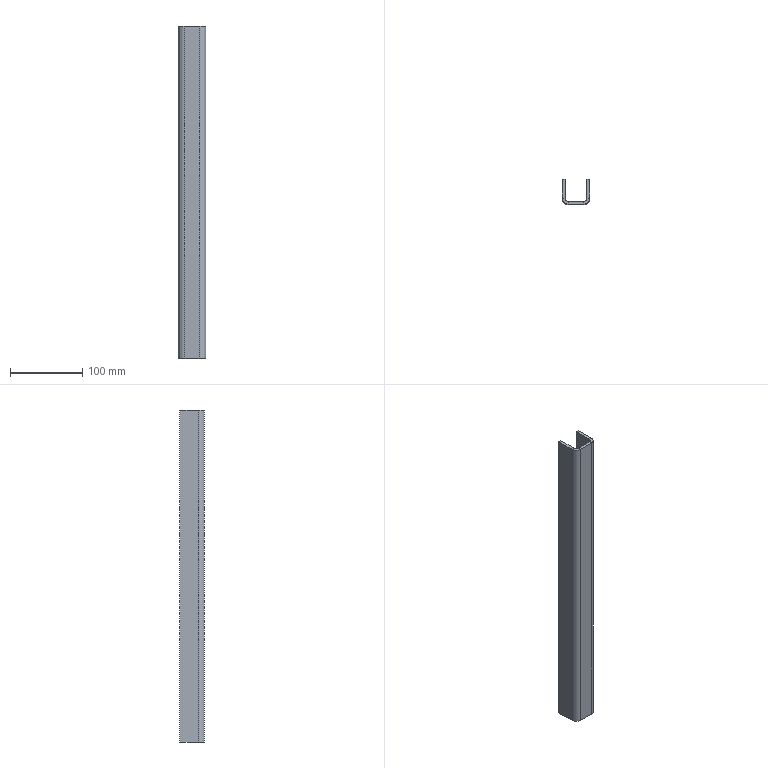Part | STEP file | 17-Reinforcing bent plate 1 | 1 solid | 22 faces | box 38 x 34 x 459 mm | volume 170472 mm3 | plane 18 | cylinder 4 | commonest cylinder face diameters 8 x2 16 x2
STEP:
#1=CARTESIAN_POINT('',(0.,0.,0.));
#2=DIRECTION('',(0.,0.,1.));
#3=DIRECTION('',(1.,0.,0.));
#4=AXIS2_PLACEMENT_3D('',#1,#2,#3);
#5=CARTESIAN_POINT('',(0.,-26.,459.));
#6=VERTEX_POINT('',#5);
#7=CARTESIAN_POINT('',(4.,-26.,459.));
#8=VERTEX_POINT('',#7);
#9=CARTESIAN_POINT('',(0.,-26.,459.));
#10=DIRECTION('',(1.,0.,0.));
#11=VECTOR('',#10,1.);
#12=LINE('',#9,#11);
#13=CARTESIAN_POINT('',(0.,-26.,459.));
#14=DIRECTION('',(0.,0.,1.));
#15=DIRECTION('',(1.,0.,0.));
#16=AXIS2_PLACEMENT_3D('',#13,#14,#15);
#17=PLANE('',#16);
#18=CARTESIAN_POINT('',(0.,0.));
#19=DIRECTION('',(1.,0.));
#20=VECTOR('',#19,1.);
#21=LINE('',#18,#20);
#22=(GEOMETRIC_REPRESENTATION_CONTEXT(2)PARAMETRIC_REPRESENTATION_CONTEXT()REPRESENTATION_CONTEXT('',''));
#23=DEFINITIONAL_REPRESENTATION('',(#21),#22);
#24=PCURVE('',#17,#23);
#25=CARTESIAN_POINT('',(8.,-30.,459.));
#26=DIRECTION('',(0.,0.,1.));
#27=DIRECTION('',(1.,0.,0.));
#28=AXIS2_PLACEMENT_3D('',#25,#26,#27);
#29=PLANE('',#28);
#30=CARTESIAN_POINT('',(-8.,4.));
#31=DIRECTION('',(1.,0.));
#32=VECTOR('',#31,1.);
#33=LINE('',#30,#32);
#34=(GEOMETRIC_REPRESENTATION_CONTEXT(2)PARAMETRIC_REPRESENTATION_CONTEXT()REPRESENTATION_CONTEXT('',''));
#35=DEFINITIONAL_REPRESENTATION('',(#33),#34);
#36=PCURVE('',#29,#35);
#37=SURFACE_CURVE('',#12,(#24,#36),.PCURVE_S1.);
#38=EDGE_CURVE('',#6,#8,#37,.T.);
#39=ORIENTED_EDGE('',*,*,#38,.F.);
#40=CARTESIAN_POINT('',(8.,-34.,459.));
#41=VERTEX_POINT('',#40);
#42=CARTESIAN_POINT('',(8.,-26.,459.));
#43=DIRECTION('',(0.,0.,1.));
#44=DIRECTION('',(-1.,0.,0.));
#45=AXIS2_PLACEMENT_3D('',#42,#43,#44);
#46=CIRCLE('',#45,8.);
#47=CARTESIAN_POINT('',(8.,0.));
#48=DIRECTION('',(-1.,0.));
#49=AXIS2_PLACEMENT_2D('',#47,#48);
#50=CIRCLE('',#49,8.);
#51=(GEOMETRIC_REPRESENTATION_CONTEXT(2)PARAMETRIC_REPRESENTATION_CONTEXT()REPRESENTATION_CONTEXT('',''));
#52=DEFINITIONAL_REPRESENTATION('',(#50),#51);
#53=PCURVE('',#17,#52);
#54=CARTESIAN_POINT('',(8.,-26.,459.));
#55=DIRECTION('',(0.,0.,-1.));
#56=DIRECTION('',(-1.,0.,0.));
#57=AXIS2_PLACEMENT_3D('',#54,#55,#56);
#58=CYLINDRICAL_SURFACE('',#57,8.);
#59=CARTESIAN_POINT('',(6.283,0.));
#60=DIRECTION('',(-1.,0.));
#61=VECTOR('',#60,1.);
#62=LINE('',#59,#61);
#63=(GEOMETRIC_REPRESENTATION_CONTEXT(2)PARAMETRIC_REPRESENTATION_CONTEXT()REPRESENTATION_CONTEXT('',''));
#64=DEFINITIONAL_REPRESENTATION('',(#62),#63);
#65=PCURVE('',#58,#64);
#66=SURFACE_CURVE('',#46,(#53,#65),.PCURVE_S1.);
#67=EDGE_CURVE('',#6,#41,#66,.T.);
#68=ORIENTED_EDGE('',*,*,#67,.T.);
#69=CARTESIAN_POINT('',(8.,-30.,459.));
#70=VERTEX_POINT('',#69);
#71=CARTESIAN_POINT('',(8.,-30.,459.));
#72=DIRECTION('',(0.,-1.,0.));
#73=VECTOR('',#72,1.);
#74=LINE('',#71,#73);
#75=CARTESIAN_POINT('',(8.,-4.));
#76=DIRECTION('',(0.,-1.));
#77=VECTOR('',#76,1.);
#78=LINE('',#75,#77);
#79=(GEOMETRIC_REPRESENTATION_CONTEXT(2)PARAMETRIC_REPRESENTATION_CONTEXT()REPRESENTATION_CONTEXT('',''));
#80=DEFINITIONAL_REPRESENTATION('',(#78),#79);
#81=PCURVE('',#17,#80);
#82=CARTESIAN_POINT('',(34.,-26.,459.));
#83=DIRECTION('',(0.,0.,1.));
#84=DIRECTION('',(1.,0.,0.));
#85=AXIS2_PLACEMENT_3D('',#82,#83,#84);
#86=PLANE('',#85);
#87=CARTESIAN_POINT('',(-26.,-4.));
#88=DIRECTION('',(0.,-1.));
#89=VECTOR('',#88,1.);
#90=LINE('',#87,#89);
#91=(GEOMETRIC_REPRESENTATION_CONTEXT(2)PARAMETRIC_REPRESENTATION_CONTEXT()REPRESENTATION_CONTEXT('',''));
#92=DEFINITIONAL_REPRESENTATION('',(#90),#91);
#93=PCURVE('',#86,#92);
#94=SURFACE_CURVE('',#74,(#81,#93),.PCURVE_S1.);
#95=EDGE_CURVE('',#70,#41,#94,.T.);
#96=ORIENTED_EDGE('',*,*,#95,.F.);
#97=CARTESIAN_POINT('',(8.,-26.,459.));
#98=DIRECTION('',(0.,0.,1.));
#99=DIRECTION('',(1.,0.,0.));
#100=AXIS2_PLACEMENT_3D('',#97,#98,#99);
#101=CIRCLE('',#100,4.);
#102=CARTESIAN_POINT('',(8.,0.));
#103=DIRECTION('',(1.,0.));
#104=AXIS2_PLACEMENT_2D('',#102,#103);
#105=CIRCLE('',#104,4.);
#106=(GEOMETRIC_REPRESENTATION_CONTEXT(2)PARAMETRIC_REPRESENTATION_CONTEXT()REPRESENTATION_CONTEXT('',''));
#107=DEFINITIONAL_REPRESENTATION('',(#105),#106);
#108=PCURVE('',#17,#107);
#109=CARTESIAN_POINT('',(8.,-26.,459.));
#110=DIRECTION('',(0.,0.,-1.));
#111=DIRECTION('',(-1.,0.,0.));
#112=AXIS2_PLACEMENT_3D('',#109,#110,#111);
#113=CYLINDRICAL_SURFACE('',#112,4.);
#114=CARTESIAN_POINT('',(9.425,0.));
#115=DIRECTION('',(-1.,0.));
#116=VECTOR('',#115,1.);
#117=LINE('',#114,#116);
#118=(GEOMETRIC_REPRESENTATION_CONTEXT(2)PARAMETRIC_REPRESENTATION_CONTEXT()REPRESENTATION_CONTEXT('',''));
#119=DEFINITIONAL_REPRESENTATION('',(#117),#118);
#120=PCURVE('',#113,#119);
#121=SURFACE_CURVE('',#101,(#108,#120),.PCURVE_S1.);
#122=EDGE_CURVE('',#8,#70,#121,.T.);
#123=ORIENTED_EDGE('',*,*,#122,.F.);
#124=EDGE_LOOP('',(#39,#68,#96,#123));
#125=FACE_BOUND('',#124,.T.);
#126=ADVANCED_FACE('',(#125),#17,.T.);
#127=CARTESIAN_POINT('',(0.,0.,459.));
#128=VERTEX_POINT('',#127);
#129=CARTESIAN_POINT('',(0.,0.,459.));
#130=DIRECTION('',(0.,-1.,0.));
#131=VECTOR('',#130,1.);
#132=LINE('',#129,#131);
#133=CARTESIAN_POINT('',(-8.,30.));
#134=DIRECTION('',(0.,-1.));
#135=VECTOR('',#134,1.);
#136=LINE('',#133,#135);
#137=(GEOMETRIC_REPRESENTATION_CONTEXT(2)PARAMETRIC_REPRESENTATION_CONTEXT()REPRESENTATION_CONTEXT('',''));
#138=DEFINITIONAL_REPRESENTATION('',(#136),#137);
#139=PCURVE('',#29,#138);
#140=CARTESIAN_POINT('',(0.,0.,459.));
#141=DIRECTION('',(1.,0.,0.));
#142=DIRECTION('',(0.,1.,0.));
#143=AXIS2_PLACEMENT_3D('',#140,#141,#142);
#144=PLANE('',#143);
#145=CARTESIAN_POINT('',(0.,0.));
#146=DIRECTION('',(-1.,0.));
#147=VECTOR('',#146,1.);
#148=LINE('',#145,#147);
#149=(GEOMETRIC_REPRESENTATION_CONTEXT(2)PARAMETRIC_REPRESENTATION_CONTEXT()REPRESENTATION_CONTEXT('',''));
#150=DEFINITIONAL_REPRESENTATION('',(#148),#149);
#151=PCURVE('',#144,#150);
#152=SURFACE_CURVE('',#132,(#139,#151),.PCURVE_S1.);
#153=EDGE_CURVE('',#128,#6,#152,.T.);
#154=ORIENTED_EDGE('',*,*,#153,.T.);
#155=ORIENTED_EDGE('',*,*,#38,.T.);
#156=CARTESIAN_POINT('',(4.,0.,459.));
#157=VERTEX_POINT('',#156);
#158=CARTESIAN_POINT('',(4.,0.,459.));
#159=DIRECTION('',(0.,-1.,0.));
#160=VECTOR('',#159,1.);
#161=LINE('',#158,#160);
#162=CARTESIAN_POINT('',(-4.,30.));
#163=DIRECTION('',(0.,-1.));
#164=VECTOR('',#163,1.);
#165=LINE('',#162,#164);
#166=(GEOMETRIC_REPRESENTATION_CONTEXT(2)PARAMETRIC_REPRESENTATION_CONTEXT()REPRESENTATION_CONTEXT('',''));
#167=DEFINITIONAL_REPRESENTATION('',(#165),#166);
#168=PCURVE('',#29,#167);
#169=CARTESIAN_POINT('',(4.,0.,459.));
#170=DIRECTION('',(1.,0.,0.));
#171=DIRECTION('',(0.,1.,0.));
#172=AXIS2_PLACEMENT_3D('',#169,#170,#171);
#173=PLANE('',#172);
#174=CARTESIAN_POINT('',(0.,0.));
#175=DIRECTION('',(-1.,0.));
#176=VECTOR('',#175,1.);
#177=LINE('',#174,#176);
#178=(GEOMETRIC_REPRESENTATION_CONTEXT(2)PARAMETRIC_REPRESENTATION_CONTEXT()REPRESENTATION_CONTEXT('',''));
#179=DEFINITIONAL_REPRESENTATION('',(#177),#178);
#180=PCURVE('',#173,#179);
#181=SURFACE_CURVE('',#161,(#168,#180),.PCURVE_S1.);
#182=EDGE_CURVE('',#157,#8,#181,.T.);
#183=ORIENTED_EDGE('',*,*,#182,.F.);
#184=CARTESIAN_POINT('',(0.,0.,459.));
#185=DIRECTION('',(1.,0.,0.));
#186=VECTOR('',#185,1.);
#187=LINE('',#184,#186);
#188=CARTESIAN_POINT('',(-8.,30.));
#189=DIRECTION('',(1.,0.));
#190=VECTOR('',#189,1.);
#191=LINE('',#188,#190);
#192=(GEOMETRIC_REPRESENTATION_CONTEXT(2)PARAMETRIC_REPRESENTATION_CONTEXT()REPRESENTATION_CONTEXT('',''));
#193=DEFINITIONAL_REPRESENTATION('',(#191),#192);
#194=PCURVE('',#29,#193);
#195=CARTESIAN_POINT('',(0.,0.,459.));
#196=DIRECTION('',(0.,1.,0.));
#197=DIRECTION('',(-1.,0.,0.));
#198=AXIS2_PLACEMENT_3D('',#195,#196,#197);
#199=PLANE('',#198);
#200=CARTESIAN_POINT('',(0.,0.));
#201=DIRECTION('',(-1.,0.));
#202=VECTOR('',#201,1.);
#203=LINE('',#200,#202);
#204=(GEOMETRIC_REPRESENTATION_CONTEXT(2)PARAMETRIC_REPRESENTATION_CONTEXT()REPRESENTATION_CONTEXT('',''));
#205=DEFINITIONAL_REPRESENTATION('',(#203),#204);
#206=PCURVE('',#199,#205);
#207=SURFACE_CURVE('',#187,(#194,#206),.PCURVE_S1.);
#208=EDGE_CURVE('',#128,#157,#207,.T.);
#209=ORIENTED_EDGE('',*,*,#208,.F.);
#210=EDGE_LOOP('',(#154,#155,#183,#209));
#211=FACE_BOUND('',#210,.T.);
#212=ADVANCED_FACE('',(#211),#29,.T.);
#213=CARTESIAN_POINT('',(8.,-34.,0.));
#214=VERTEX_POINT('',#213);
#215=CARTESIAN_POINT('',(8.,-30.,0.));
#216=VERTEX_POINT('',#215);
#217=CARTESIAN_POINT('',(8.,-34.,0.));
#218=DIRECTION('',(0.,1.,0.));
#219=VECTOR('',#218,1.);
#220=LINE('',#217,#219);
#221=CARTESIAN_POINT('',(8.,-34.,0.));
#222=DIRECTION('',(0.,0.,-1.));
#223=DIRECTION('',(-1.,0.,0.));
#224=AXIS2_PLACEMENT_3D('',#221,#222,#223);
#225=PLANE('',#224);
#226=CARTESIAN_POINT('',(0.,0.));
#227=DIRECTION('',(0.,1.));
#228=VECTOR('',#227,1.);
#229=LINE('',#226,#228);
#230=(GEOMETRIC_REPRESENTATION_CONTEXT(2)PARAMETRIC_REPRESENTATION_CONTEXT()REPRESENTATION_CONTEXT('',''));
#231=DEFINITIONAL_REPRESENTATION('',(#229),#230);
#232=PCURVE('',#225,#231);
#233=CARTESIAN_POINT('',(4.,-26.,0.));
#234=DIRECTION('',(0.,0.,-1.));
#235=DIRECTION('',(-1.,0.,0.));
#236=AXIS2_PLACEMENT_3D('',#233,#234,#235);
#237=PLANE('',#236);
#238=CARTESIAN_POINT('',(-4.,-8.));
#239=DIRECTION('',(0.,1.));
#240=VECTOR('',#239,1.);
#241=LINE('',#238,#240);
#242=(GEOMETRIC_REPRESENTATION_CONTEXT(2)PARAMETRIC_REPRESENTATION_CONTEXT()REPRESENTATION_CONTEXT('',''));
#243=DEFINITIONAL_REPRESENTATION('',(#241),#242);
#244=PCURVE('',#237,#243);
#245=SURFACE_CURVE('',#220,(#232,#244),.PCURVE_S1.);
#246=EDGE_CURVE('',#214,#216,#245,.T.);
#247=ORIENTED_EDGE('',*,*,#246,.F.);
#248=CARTESIAN_POINT('',(0.,-26.,0.));
#249=VERTEX_POINT('',#248);
#250=CARTESIAN_POINT('',(8.,-26.,0.));
#251=DIRECTION('',(0.,0.,1.));
#252=DIRECTION('',(-1.,0.,0.));
#253=AXIS2_PLACEMENT_3D('',#250,#251,#252);
#254=CIRCLE('',#253,8.);
#255=CARTESIAN_POINT('',(8.,8.));
#256=CARTESIAN_POINT('',(8.,-5.856));
#257=CARTESIAN_POINT('',(-4.,1.072));
#258=CARTESIAN_POINT('',(-16.,8.));
#259=CARTESIAN_POINT('',(-4.,14.928));
#260=CARTESIAN_POINT('',(8.,21.856));
#261=CARTESIAN_POINT('',(8.,8.));
#262=(BOUNDED_CURVE()B_SPLINE_CURVE(2,(#255,#256,#257,#258,#259,#260,#261),.UNSPECIFIED.,.T.,.F.)B_SPLINE_CURVE_WITH_KNOTS((1,2,2,2,2,1),(-2.094,0.,2.094,4.189,6.283,8.378),.UNSPECIFIED.)CURVE()GEOMETRIC_REPRESENTATION_ITEM()RATIONAL_B_SPLINE_CURVE((1.,0.5,1.,0.5,1.,0.5,1.))REPRESENTATION_ITEM(''));
#263=(GEOMETRIC_REPRESENTATION_CONTEXT(2)PARAMETRIC_REPRESENTATION_CONTEXT()REPRESENTATION_CONTEXT('',''));
#264=DEFINITIONAL_REPRESENTATION('',(#262),#263);
#265=PCURVE('',#225,#264);
#266=CARTESIAN_POINT('',(6.283,459.));
#267=DIRECTION('',(-1.,0.));
#268=VECTOR('',#267,1.);
#269=LINE('',#266,#268);
#270=(GEOMETRIC_REPRESENTATION_CONTEXT(2)PARAMETRIC_REPRESENTATION_CONTEXT()REPRESENTATION_CONTEXT('',''));
#271=DEFINITIONAL_REPRESENTATION('',(#269),#270);
#272=PCURVE('',#58,#271);
#273=SURFACE_CURVE('',#254,(#265,#272),.PCURVE_S1.);
#274=EDGE_CURVE('',#249,#214,#273,.T.);
#275=ORIENTED_EDGE('',*,*,#274,.F.);
#276=CARTESIAN_POINT('',(4.,-26.,0.));
#277=VERTEX_POINT('',#276);
#278=CARTESIAN_POINT('',(4.,-26.,0.));
#279=DIRECTION('',(-1.,0.,0.));
#280=VECTOR('',#279,1.);
#281=LINE('',#278,#280);
#282=CARTESIAN_POINT('',(4.,8.));
#283=DIRECTION('',(1.,0.));
#284=VECTOR('',#283,1.);
#285=LINE('',#282,#284);
#286=(GEOMETRIC_REPRESENTATION_CONTEXT(2)PARAMETRIC_REPRESENTATION_CONTEXT()REPRESENTATION_CONTEXT('',''));
#287=DEFINITIONAL_REPRESENTATION('',(#285),#286);
#288=PCURVE('',#225,#287);
#289=CARTESIAN_POINT('',(30.,-26.,0.));
#290=DIRECTION('',(0.,0.,1.));
#291=DIRECTION('',(1.,0.,0.));
#292=AXIS2_PLACEMENT_3D('',#289,#290,#291);
#293=PLANE('',#292);
#294=CARTESIAN_POINT('',(-26.,0.));
#295=DIRECTION('',(-1.,0.));
#296=VECTOR('',#295,1.);
#297=LINE('',#294,#296);
#298=(GEOMETRIC_REPRESENTATION_CONTEXT(2)PARAMETRIC_REPRESENTATION_CONTEXT()REPRESENTATION_CONTEXT('',''));
#299=DEFINITIONAL_REPRESENTATION('',(#297),#298);
#300=PCURVE('',#293,#299);
#301=SURFACE_CURVE('',#281,(#288,#300),.PCURVE_S1.);
#302=EDGE_CURVE('',#277,#249,#301,.T.);
#303=ORIENTED_EDGE('',*,*,#302,.F.);
#304=CARTESIAN_POINT('',(8.,-26.,0.));
#305=DIRECTION('',(0.,0.,1.));
#306=DIRECTION('',(1.,0.,0.));
#307=AXIS2_PLACEMENT_3D('',#304,#305,#306);
#308=CIRCLE('',#307,4.);
#309=CARTESIAN_POINT('',(-4.,8.));
#310=CARTESIAN_POINT('',(-4.,14.928));
#311=CARTESIAN_POINT('',(2.,11.464));
#312=CARTESIAN_POINT('',(8.,8.));
#313=CARTESIAN_POINT('',(2.,4.536));
#314=CARTESIAN_POINT('',(-4.,1.072));
#315=CARTESIAN_POINT('',(-4.,8.));
#316=(BOUNDED_CURVE()B_SPLINE_CURVE(2,(#309,#310,#311,#312,#313,#314,#315),.UNSPECIFIED.,.T.,.F.)B_SPLINE_CURVE_WITH_KNOTS((1,2,2,2,2,1),(-2.094,0.,2.094,4.189,6.283,8.378),.UNSPECIFIED.)CURVE()GEOMETRIC_REPRESENTATION_ITEM()RATIONAL_B_SPLINE_CURVE((1.,0.5,1.,0.5,1.,0.5,1.))REPRESENTATION_ITEM(''));
#317=(GEOMETRIC_REPRESENTATION_CONTEXT(2)PARAMETRIC_REPRESENTATION_CONTEXT()REPRESENTATION_CONTEXT('',''));
#318=DEFINITIONAL_REPRESENTATION('',(#316),#317);
#319=PCURVE('',#225,#318);
#320=CARTESIAN_POINT('',(9.425,459.));
#321=DIRECTION('',(-1.,0.));
#322=VECTOR('',#321,1.);
#323=LINE('',#320,#322);
#324=(GEOMETRIC_REPRESENTATION_CONTEXT(2)PARAMETRIC_REPRESENTATION_CONTEXT()REPRESENTATION_CONTEXT('',''));
#325=DEFINITIONAL_REPRESENTATION('',(#323),#324);
#326=PCURVE('',#113,#325);
#327=SURFACE_CURVE('',#308,(#319,#326),.PCURVE_S1.);
#328=EDGE_CURVE('',#277,#216,#327,.T.);
#329=ORIENTED_EDGE('',*,*,#328,.T.);
#330=EDGE_LOOP('',(#247,#275,#303,#329));
#331=FACE_BOUND('',#330,.T.);
#332=ADVANCED_FACE('',(#331),#225,.T.);
#333=CARTESIAN_POINT('',(30.,-34.,0.));
#334=VERTEX_POINT('',#333);
#335=CARTESIAN_POINT('',(0.,-34.,0.));
#336=DIRECTION('',(1.,0.,0.));
#337=VECTOR('',#336,1.);
#338=LINE('',#335,#337);
#339=CARTESIAN_POINT('',(4.,-8.));
#340=DIRECTION('',(-1.,0.));
#341=VECTOR('',#340,1.);
#342=LINE('',#339,#341);
#343=(GEOMETRIC_REPRESENTATION_CONTEXT(2)PARAMETRIC_REPRESENTATION_CONTEXT()REPRESENTATION_CONTEXT('',''));
#344=DEFINITIONAL_REPRESENTATION('',(#342),#343);
#345=PCURVE('',#237,#344);
#346=CARTESIAN_POINT('',(0.,-34.,459.));
#347=DIRECTION('',(0.,1.,0.));
#348=DIRECTION('',(0.,0.,1.));
#349=AXIS2_PLACEMENT_3D('',#346,#347,#348);
#350=PLANE('',#349);
#351=CARTESIAN_POINT('',(-459.,0.));
#352=DIRECTION('',(0.,1.));
#353=VECTOR('',#352,1.);
#354=LINE('',#351,#353);
#355=(GEOMETRIC_REPRESENTATION_CONTEXT(2)PARAMETRIC_REPRESENTATION_CONTEXT()REPRESENTATION_CONTEXT('',''));
#356=DEFINITIONAL_REPRESENTATION('',(#354),#355);
#357=PCURVE('',#350,#356);
#358=SURFACE_CURVE('',#338,(#345,#357),.PCURVE_S1.);
#359=EDGE_CURVE('',#214,#334,#358,.T.);
#360=ORIENTED_EDGE('',*,*,#359,.F.);
#361=ORIENTED_EDGE('',*,*,#246,.T.);
#362=CARTESIAN_POINT('',(30.,-30.,0.));
#363=VERTEX_POINT('',#362);
#364=CARTESIAN_POINT('',(0.,-30.,0.));
#365=DIRECTION('',(1.,0.,0.));
#366=VECTOR('',#365,1.);
#367=LINE('',#364,#366);
#368=CARTESIAN_POINT('',(4.,-4.));
#369=DIRECTION('',(-1.,0.));
#370=VECTOR('',#369,1.);
#371=LINE('',#368,#370);
#372=(GEOMETRIC_REPRESENTATION_CONTEXT(2)PARAMETRIC_REPRESENTATION_CONTEXT()REPRESENTATION_CONTEXT('',''));
#373=DEFINITIONAL_REPRESENTATION('',(#371),#372);
#374=PCURVE('',#237,#373);
#375=CARTESIAN_POINT('',(0.,-30.,459.));
#376=DIRECTION('',(0.,1.,0.));
#377=DIRECTION('',(0.,0.,1.));
#378=AXIS2_PLACEMENT_3D('',#375,#376,#377);
#379=PLANE('',#378);
#380=CARTESIAN_POINT('',(-459.,0.));
#381=DIRECTION('',(0.,1.));
#382=VECTOR('',#381,1.);
#383=LINE('',#380,#382);
#384=(GEOMETRIC_REPRESENTATION_CONTEXT(2)PARAMETRIC_REPRESENTATION_CONTEXT()REPRESENTATION_CONTEXT('',''));
#385=DEFINITIONAL_REPRESENTATION('',(#383),#384);
#386=PCURVE('',#379,#385);
#387=SURFACE_CURVE('',#367,(#374,#386),.PCURVE_S1.);
#388=EDGE_CURVE('',#216,#363,#387,.T.);
#389=ORIENTED_EDGE('',*,*,#388,.T.);
#390=CARTESIAN_POINT('',(30.,-30.,0.));
#391=DIRECTION('',(0.,-1.,0.));
#392=VECTOR('',#391,1.);
#393=LINE('',#390,#392);
#394=CARTESIAN_POINT('',(-26.,-4.));
#395=DIRECTION('',(0.,-1.));
#396=VECTOR('',#395,1.);
#397=LINE('',#394,#396);
#398=(GEOMETRIC_REPRESENTATION_CONTEXT(2)PARAMETRIC_REPRESENTATION_CONTEXT()REPRESENTATION_CONTEXT('',''));
#399=DEFINITIONAL_REPRESENTATION('',(#397),#398);
#400=PCURVE('',#237,#399);
#401=CARTESIAN_POINT('',(38.,-26.,0.));
#402=DIRECTION('',(0.,0.,-1.));
#403=DIRECTION('',(-1.,0.,0.));
#404=AXIS2_PLACEMENT_3D('',#401,#402,#403);
#405=PLANE('',#404);
#406=CARTESIAN_POINT('',(8.,-4.));
#407=DIRECTION('',(0.,-1.));
#408=VECTOR('',#407,1.);
#409=LINE('',#406,#408);
#410=(GEOMETRIC_REPRESENTATION_CONTEXT(2)PARAMETRIC_REPRESENTATION_CONTEXT()REPRESENTATION_CONTEXT('',''));
#411=DEFINITIONAL_REPRESENTATION('',(#409),#410);
#412=PCURVE('',#405,#411);
#413=SURFACE_CURVE('',#393,(#400,#412),.PCURVE_S1.);
#414=EDGE_CURVE('',#363,#334,#413,.T.);
#415=ORIENTED_EDGE('',*,*,#414,.T.);
#416=EDGE_LOOP('',(#360,#361,#389,#415));
#417=FACE_BOUND('',#416,.T.);
#418=ADVANCED_FACE('',(#417),#237,.T.);
#419=CARTESIAN_POINT('',(30.,-34.,459.));
#420=VERTEX_POINT('',#419);
#421=CARTESIAN_POINT('',(30.,-30.,459.));
#422=VERTEX_POINT('',#421);
#423=CARTESIAN_POINT('',(30.,-34.,459.));
#424=DIRECTION('',(0.,1.,0.));
#425=VECTOR('',#424,1.);
#426=LINE('',#423,#425);
#427=CARTESIAN_POINT('',(30.,-34.,459.));
#428=DIRECTION('',(0.,0.,1.));
#429=DIRECTION('',(1.,0.,0.));
#430=AXIS2_PLACEMENT_3D('',#427,#428,#429);
#431=PLANE('',#430);
#432=CARTESIAN_POINT('',(0.,0.));
#433=DIRECTION('',(0.,1.));
#434=VECTOR('',#433,1.);
#435=LINE('',#432,#434);
#436=(GEOMETRIC_REPRESENTATION_CONTEXT(2)PARAMETRIC_REPRESENTATION_CONTEXT()REPRESENTATION_CONTEXT('',''));
#437=DEFINITIONAL_REPRESENTATION('',(#435),#436);
#438=PCURVE('',#431,#437);
#439=CARTESIAN_POINT('',(-4.,-8.));
#440=DIRECTION('',(0.,1.));
#441=VECTOR('',#440,1.);
#442=LINE('',#439,#441);
#443=(GEOMETRIC_REPRESENTATION_CONTEXT(2)PARAMETRIC_REPRESENTATION_CONTEXT()REPRESENTATION_CONTEXT('',''));
#444=DEFINITIONAL_REPRESENTATION('',(#442),#443);
#445=PCURVE('',#86,#444);
#446=SURFACE_CURVE('',#426,(#438,#445),.PCURVE_S1.);
#447=EDGE_CURVE('',#420,#422,#446,.T.);
#448=ORIENTED_EDGE('',*,*,#447,.F.);
#449=CARTESIAN_POINT('',(38.,-26.,459.));
#450=VERTEX_POINT('',#449);
#451=CARTESIAN_POINT('',(30.,-26.,459.));
#452=DIRECTION('',(0.,0.,1.));
#453=DIRECTION('',(-1.,0.,0.));
#454=AXIS2_PLACEMENT_3D('',#451,#452,#453);
#455=CIRCLE('',#454,8.);
#456=CARTESIAN_POINT('',(0.,8.));
#457=DIRECTION('',(-1.,0.));
#458=AXIS2_PLACEMENT_2D('',#456,#457);
#459=CIRCLE('',#458,8.);
#460=(GEOMETRIC_REPRESENTATION_CONTEXT(2)PARAMETRIC_REPRESENTATION_CONTEXT()REPRESENTATION_CONTEXT('',''));
#461=DEFINITIONAL_REPRESENTATION('',(#459),#460);
#462=PCURVE('',#431,#461);
#463=CARTESIAN_POINT('',(30.,-26.,459.));
#464=DIRECTION('',(0.,0.,-1.));
#465=DIRECTION('',(-1.,0.,0.));
#466=AXIS2_PLACEMENT_3D('',#463,#464,#465);
#467=CYLINDRICAL_SURFACE('',#466,8.);
#468=CARTESIAN_POINT('',(6.283,0.));
#469=DIRECTION('',(-1.,0.));
#470=VECTOR('',#469,1.);
#471=LINE('',#468,#470);
#472=(GEOMETRIC_REPRESENTATION_CONTEXT(2)PARAMETRIC_REPRESENTATION_CONTEXT()REPRESENTATION_CONTEXT('',''));
#473=DEFINITIONAL_REPRESENTATION('',(#471),#472);
#474=PCURVE('',#467,#473);
#475=SURFACE_CURVE('',#455,(#462,#474),.PCURVE_S1.);
#476=EDGE_CURVE('',#420,#450,#475,.T.);
#477=ORIENTED_EDGE('',*,*,#476,.T.);
#478=CARTESIAN_POINT('',(34.,-26.,459.));
#479=VERTEX_POINT('',#478);
#480=CARTESIAN_POINT('',(34.,-26.,459.));
#481=DIRECTION('',(1.,0.,0.));
#482=VECTOR('',#481,1.);
#483=LINE('',#480,#482);
#484=CARTESIAN_POINT('',(4.,8.));
#485=DIRECTION('',(1.,0.));
#486=VECTOR('',#485,1.);
#487=LINE('',#484,#486);
#488=(GEOMETRIC_REPRESENTATION_CONTEXT(2)PARAMETRIC_REPRESENTATION_CONTEXT()REPRESENTATION_CONTEXT('',''));
#489=DEFINITIONAL_REPRESENTATION('',(#487),#488);
#490=PCURVE('',#431,#489);
#491=CARTESIAN_POINT('',(30.,-26.,459.));
#492=DIRECTION('',(0.,0.,1.));
#493=DIRECTION('',(1.,0.,0.));
#494=AXIS2_PLACEMENT_3D('',#491,#492,#493);
#495=PLANE('',#494);
#496=CARTESIAN_POINT('',(4.,0.));
#497=DIRECTION('',(1.,0.));
#498=VECTOR('',#497,1.);
#499=LINE('',#496,#498);
#500=(GEOMETRIC_REPRESENTATION_CONTEXT(2)PARAMETRIC_REPRESENTATION_CONTEXT()REPRESENTATION_CONTEXT('',''));
#501=DEFINITIONAL_REPRESENTATION('',(#499),#500);
#502=PCURVE('',#495,#501);
#503=SURFACE_CURVE('',#483,(#490,#502),.PCURVE_S1.);
#504=EDGE_CURVE('',#479,#450,#503,.T.);
#505=ORIENTED_EDGE('',*,*,#504,.F.);
#506=CARTESIAN_POINT('',(30.,-26.,459.));
#507=DIRECTION('',(0.,0.,1.));
#508=DIRECTION('',(1.,0.,0.));
#509=AXIS2_PLACEMENT_3D('',#506,#507,#508);
#510=CIRCLE('',#509,4.);
#511=CARTESIAN_POINT('',(0.,8.));
#512=DIRECTION('',(1.,0.));
#513=AXIS2_PLACEMENT_2D('',#511,#512);
#514=CIRCLE('',#513,4.);
#515=(GEOMETRIC_REPRESENTATION_CONTEXT(2)PARAMETRIC_REPRESENTATION_CONTEXT()REPRESENTATION_CONTEXT('',''));
#516=DEFINITIONAL_REPRESENTATION('',(#514),#515);
#517=PCURVE('',#431,#516);
#518=CARTESIAN_POINT('',(30.,-26.,459.));
#519=DIRECTION('',(0.,0.,-1.));
#520=DIRECTION('',(-1.,0.,0.));
#521=AXIS2_PLACEMENT_3D('',#518,#519,#520);
#522=CYLINDRICAL_SURFACE('',#521,4.);
#523=CARTESIAN_POINT('',(9.425,0.));
#524=DIRECTION('',(-1.,0.));
#525=VECTOR('',#524,1.);
#526=LINE('',#523,#525);
#527=(GEOMETRIC_REPRESENTATION_CONTEXT(2)PARAMETRIC_REPRESENTATION_CONTEXT()REPRESENTATION_CONTEXT('',''));
#528=DEFINITIONAL_REPRESENTATION('',(#526),#527);
#529=PCURVE('',#522,#528);
#530=SURFACE_CURVE('',#510,(#517,#529),.PCURVE_S1.);
#531=EDGE_CURVE('',#422,#479,#530,.T.);
#532=ORIENTED_EDGE('',*,*,#531,.F.);
#533=EDGE_LOOP('',(#448,#477,#505,#532));
#534=FACE_BOUND('',#533,.T.);
#535=ADVANCED_FACE('',(#534),#431,.T.);
#536=CARTESIAN_POINT('',(0.,-34.,459.));
#537=DIRECTION('',(1.,0.,0.));
#538=VECTOR('',#537,1.);
#539=LINE('',#536,#538);
#540=CARTESIAN_POINT('',(-34.,-8.));
#541=DIRECTION('',(1.,0.));
#542=VECTOR('',#541,1.);
#543=LINE('',#540,#542);
#544=(GEOMETRIC_REPRESENTATION_CONTEXT(2)PARAMETRIC_REPRESENTATION_CONTEXT()REPRESENTATION_CONTEXT('',''));
#545=DEFINITIONAL_REPRESENTATION('',(#543),#544);
#546=PCURVE('',#86,#545);
#547=CARTESIAN_POINT('',(0.,0.));
#548=DIRECTION('',(0.,1.));
#549=VECTOR('',#548,1.);
#550=LINE('',#547,#549);
#551=(GEOMETRIC_REPRESENTATION_CONTEXT(2)PARAMETRIC_REPRESENTATION_CONTEXT()REPRESENTATION_CONTEXT('',''));
#552=DEFINITIONAL_REPRESENTATION('',(#550),#551);
#553=PCURVE('',#350,#552);
#554=SURFACE_CURVE('',#539,(#546,#553),.PCURVE_S1.);
#555=EDGE_CURVE('',#41,#420,#554,.T.);
#556=ORIENTED_EDGE('',*,*,#555,.T.);
#557=ORIENTED_EDGE('',*,*,#447,.T.);
#558=CARTESIAN_POINT('',(0.,-30.,459.));
#559=DIRECTION('',(1.,0.,0.));
#560=VECTOR('',#559,1.);
#561=LINE('',#558,#560);
#562=CARTESIAN_POINT('',(-34.,-4.));
#563=DIRECTION('',(1.,0.));
#564=VECTOR('',#563,1.);
#565=LINE('',#562,#564);
#566=(GEOMETRIC_REPRESENTATION_CONTEXT(2)PARAMETRIC_REPRESENTATION_CONTEXT()REPRESENTATION_CONTEXT('',''));
#567=DEFINITIONAL_REPRESENTATION('',(#565),#566);
#568=PCURVE('',#86,#567);
#569=CARTESIAN_POINT('',(0.,0.));
#570=DIRECTION('',(0.,1.));
#571=VECTOR('',#570,1.);
#572=LINE('',#569,#571);
#573=(GEOMETRIC_REPRESENTATION_CONTEXT(2)PARAMETRIC_REPRESENTATION_CONTEXT()REPRESENTATION_CONTEXT('',''));
#574=DEFINITIONAL_REPRESENTATION('',(#572),#573);
#575=PCURVE('',#379,#574);
#576=SURFACE_CURVE('',#561,(#568,#575),.PCURVE_S1.);
#577=EDGE_CURVE('',#70,#422,#576,.T.);
#578=ORIENTED_EDGE('',*,*,#577,.F.);
#579=ORIENTED_EDGE('',*,*,#95,.T.);
#580=EDGE_LOOP('',(#556,#557,#578,#579));
#581=FACE_BOUND('',#580,.T.);
#582=ADVANCED_FACE('',(#581),#86,.T.);
#583=CARTESIAN_POINT('',(38.,-26.,0.));
#584=VERTEX_POINT('',#583);
#585=CARTESIAN_POINT('',(34.,-26.,0.));
#586=VERTEX_POINT('',#585);
#587=CARTESIAN_POINT('',(38.,-26.,0.));
#588=DIRECTION('',(-1.,0.,0.));
#589=VECTOR('',#588,1.);
#590=LINE('',#587,#589);
#591=CARTESIAN_POINT('',(0.,0.));
#592=DIRECTION('',(1.,0.));
#593=VECTOR('',#592,1.);
#594=LINE('',#591,#593);
#595=(GEOMETRIC_REPRESENTATION_CONTEXT(2)PARAMETRIC_REPRESENTATION_CONTEXT()REPRESENTATION_CONTEXT('',''));
#596=DEFINITIONAL_REPRESENTATION('',(#594),#595);
#597=PCURVE('',#405,#596);
#598=CARTESIAN_POINT('',(30.,-30.,0.));
#599=DIRECTION('',(0.,0.,-1.));
#600=DIRECTION('',(-1.,0.,0.));
#601=AXIS2_PLACEMENT_3D('',#598,#599,#600);
#602=PLANE('',#601);
#603=CARTESIAN_POINT('',(-8.,4.));
#604=DIRECTION('',(1.,0.));
#605=VECTOR('',#604,1.);
#606=LINE('',#603,#605);
#607=(GEOMETRIC_REPRESENTATION_CONTEXT(2)PARAMETRIC_REPRESENTATION_CONTEXT()REPRESENTATION_CONTEXT('',''));
#608=DEFINITIONAL_REPRESENTATION('',(#606),#607);
#609=PCURVE('',#602,#608);
#610=SURFACE_CURVE('',#590,(#597,#609),.PCURVE_S1.);
#611=EDGE_CURVE('',#584,#586,#610,.T.);
#612=ORIENTED_EDGE('',*,*,#611,.F.);
#613=CARTESIAN_POINT('',(30.,-26.,0.));
#614=DIRECTION('',(0.,0.,1.));
#615=DIRECTION('',(-1.,0.,0.));
#616=AXIS2_PLACEMENT_3D('',#613,#614,#615);
#617=CIRCLE('',#616,8.);
#618=CARTESIAN_POINT('',(16.,0.));
#619=CARTESIAN_POINT('',(16.,-13.856));
#620=CARTESIAN_POINT('',(4.,-6.928));
#621=CARTESIAN_POINT('',(-8.,0.));
#622=CARTESIAN_POINT('',(4.,6.928));
#623=CARTESIAN_POINT('',(16.,13.856));
#624=CARTESIAN_POINT('',(16.,0.));
#625=(BOUNDED_CURVE()B_SPLINE_CURVE(2,(#618,#619,#620,#621,#622,#623,#624),.UNSPECIFIED.,.T.,.F.)B_SPLINE_CURVE_WITH_KNOTS((1,2,2,2,2,1),(-2.094,0.,2.094,4.189,6.283,8.378),.UNSPECIFIED.)CURVE()GEOMETRIC_REPRESENTATION_ITEM()RATIONAL_B_SPLINE_CURVE((1.,0.5,1.,0.5,1.,0.5,1.))REPRESENTATION_ITEM(''));
#626=(GEOMETRIC_REPRESENTATION_CONTEXT(2)PARAMETRIC_REPRESENTATION_CONTEXT()REPRESENTATION_CONTEXT('',''));
#627=DEFINITIONAL_REPRESENTATION('',(#625),#626);
#628=PCURVE('',#405,#627);
#629=CARTESIAN_POINT('',(6.283,459.));
#630=DIRECTION('',(-1.,0.));
#631=VECTOR('',#630,1.);
#632=LINE('',#629,#631);
#633=(GEOMETRIC_REPRESENTATION_CONTEXT(2)PARAMETRIC_REPRESENTATION_CONTEXT()REPRESENTATION_CONTEXT('',''));
#634=DEFINITIONAL_REPRESENTATION('',(#632),#633);
#635=PCURVE('',#467,#634);
#636=SURFACE_CURVE('',#617,(#628,#635),.PCURVE_S1.);
#637=EDGE_CURVE('',#334,#584,#636,.T.);
#638=ORIENTED_EDGE('',*,*,#637,.F.);
#639=ORIENTED_EDGE('',*,*,#414,.F.);
#640=CARTESIAN_POINT('',(30.,-26.,0.));
#641=DIRECTION('',(0.,0.,1.));
#642=DIRECTION('',(1.,0.,0.));
#643=AXIS2_PLACEMENT_3D('',#640,#641,#642);
#644=CIRCLE('',#643,4.);
#645=CARTESIAN_POINT('',(4.,0.));
#646=CARTESIAN_POINT('',(4.,6.928));
#647=CARTESIAN_POINT('',(10.,3.464));
#648=CARTESIAN_POINT('',(16.,0.));
#649=CARTESIAN_POINT('',(10.,-3.464));
#650=CARTESIAN_POINT('',(4.,-6.928));
#651=CARTESIAN_POINT('',(4.,0.));
#652=(BOUNDED_CURVE()B_SPLINE_CURVE(2,(#645,#646,#647,#648,#649,#650,#651),.UNSPECIFIED.,.T.,.F.)B_SPLINE_CURVE_WITH_KNOTS((1,2,2,2,2,1),(-2.094,0.,2.094,4.189,6.283,8.378),.UNSPECIFIED.)CURVE()GEOMETRIC_REPRESENTATION_ITEM()RATIONAL_B_SPLINE_CURVE((1.,0.5,1.,0.5,1.,0.5,1.))REPRESENTATION_ITEM(''));
#653=(GEOMETRIC_REPRESENTATION_CONTEXT(2)PARAMETRIC_REPRESENTATION_CONTEXT()REPRESENTATION_CONTEXT('',''));
#654=DEFINITIONAL_REPRESENTATION('',(#652),#653);
#655=PCURVE('',#405,#654);
#656=CARTESIAN_POINT('',(9.425,459.));
#657=DIRECTION('',(-1.,0.));
#658=VECTOR('',#657,1.);
#659=LINE('',#656,#658);
#660=(GEOMETRIC_REPRESENTATION_CONTEXT(2)PARAMETRIC_REPRESENTATION_CONTEXT()REPRESENTATION_CONTEXT('',''));
#661=DEFINITIONAL_REPRESENTATION('',(#659),#660);
#662=PCURVE('',#522,#661);
#663=SURFACE_CURVE('',#644,(#655,#662),.PCURVE_S1.);
#664=EDGE_CURVE('',#363,#586,#663,.T.);
#665=ORIENTED_EDGE('',*,*,#664,.T.);
#666=EDGE_LOOP('',(#612,#638,#639,#665));
#667=FACE_BOUND('',#666,.T.);
#668=ADVANCED_FACE('',(#667),#405,.T.);
#669=CARTESIAN_POINT('',(38.,0.,0.));
#670=VERTEX_POINT('',#669);
#671=CARTESIAN_POINT('',(38.,-34.,0.));
#672=DIRECTION('',(0.,1.,0.));
#673=VECTOR('',#672,1.);
#674=LINE('',#671,#673);
#675=CARTESIAN_POINT('',(-8.,-4.));
#676=DIRECTION('',(0.,1.));
#677=VECTOR('',#676,1.);
#678=LINE('',#675,#677);
#679=(GEOMETRIC_REPRESENTATION_CONTEXT(2)PARAMETRIC_REPRESENTATION_CONTEXT()REPRESENTATION_CONTEXT('',''));
#680=DEFINITIONAL_REPRESENTATION('',(#678),#679);
#681=PCURVE('',#602,#680);
#682=CARTESIAN_POINT('',(38.,-34.,459.));
#683=DIRECTION('',(-1.,0.,0.));
#684=DIRECTION('',(0.,0.,1.));
#685=AXIS2_PLACEMENT_3D('',#682,#683,#684);
#686=PLANE('',#685);
#687=CARTESIAN_POINT('',(-459.,0.));
#688=DIRECTION('',(0.,1.));
#689=VECTOR('',#688,1.);
#690=LINE('',#687,#689);
#691=(GEOMETRIC_REPRESENTATION_CONTEXT(2)PARAMETRIC_REPRESENTATION_CONTEXT()REPRESENTATION_CONTEXT('',''));
#692=DEFINITIONAL_REPRESENTATION('',(#690),#691);
#693=PCURVE('',#686,#692);
#694=SURFACE_CURVE('',#674,(#681,#693),.PCURVE_S1.);
#695=EDGE_CURVE('',#584,#670,#694,.T.);
#696=ORIENTED_EDGE('',*,*,#695,.F.);
#697=ORIENTED_EDGE('',*,*,#611,.T.);
#698=CARTESIAN_POINT('',(34.,0.,0.));
#699=VERTEX_POINT('',#698);
#700=CARTESIAN_POINT('',(34.,-34.,0.));
#701=DIRECTION('',(0.,1.,0.));
#702=VECTOR('',#701,1.);
#703=LINE('',#700,#702);
#704=CARTESIAN_POINT('',(-4.,-4.));
#705=DIRECTION('',(0.,1.));
#706=VECTOR('',#705,1.);
#707=LINE('',#704,#706);
#708=(GEOMETRIC_REPRESENTATION_CONTEXT(2)PARAMETRIC_REPRESENTATION_CONTEXT()REPRESENTATION_CONTEXT('',''));
#709=DEFINITIONAL_REPRESENTATION('',(#707),#708);
#710=PCURVE('',#602,#709);
#711=CARTESIAN_POINT('',(34.,-34.,459.));
#712=DIRECTION('',(-1.,0.,0.));
#713=DIRECTION('',(0.,0.,1.));
#714=AXIS2_PLACEMENT_3D('',#711,#712,#713);
#715=PLANE('',#714);
#716=CARTESIAN_POINT('',(-459.,0.));
#717=DIRECTION('',(0.,1.));
#718=VECTOR('',#717,1.);
#719=LINE('',#716,#718);
#720=(GEOMETRIC_REPRESENTATION_CONTEXT(2)PARAMETRIC_REPRESENTATION_CONTEXT()REPRESENTATION_CONTEXT('',''));
#721=DEFINITIONAL_REPRESENTATION('',(#719),#720);
#722=PCURVE('',#715,#721);
#723=SURFACE_CURVE('',#703,(#710,#722),.PCURVE_S1.);
#724=EDGE_CURVE('',#586,#699,#723,.T.);
#725=ORIENTED_EDGE('',*,*,#724,.T.);
#726=CARTESIAN_POINT('',(34.,0.,0.));
#727=DIRECTION('',(1.,0.,0.));
#728=VECTOR('',#727,1.);
#729=LINE('',#726,#728);
#730=CARTESIAN_POINT('',(-4.,30.));
#731=DIRECTION('',(-1.,0.));
#732=VECTOR('',#731,1.);
#733=LINE('',#730,#732);
#734=(GEOMETRIC_REPRESENTATION_CONTEXT(2)PARAMETRIC_REPRESENTATION_CONTEXT()REPRESENTATION_CONTEXT('',''));
#735=DEFINITIONAL_REPRESENTATION('',(#733),#734);
#736=PCURVE('',#602,#735);
#737=CARTESIAN_POINT('',(34.,0.,459.));
#738=DIRECTION('',(0.,1.,0.));
#739=DIRECTION('',(0.,0.,1.));
#740=AXIS2_PLACEMENT_3D('',#737,#738,#739);
#741=PLANE('',#740);
#742=CARTESIAN_POINT('',(-459.,0.));
#743=DIRECTION('',(0.,1.));
#744=VECTOR('',#743,1.);
#745=LINE('',#742,#744);
#746=(GEOMETRIC_REPRESENTATION_CONTEXT(2)PARAMETRIC_REPRESENTATION_CONTEXT()REPRESENTATION_CONTEXT('',''));
#747=DEFINITIONAL_REPRESENTATION('',(#745),#746);
#748=PCURVE('',#741,#747);
#749=SURFACE_CURVE('',#729,(#736,#748),.PCURVE_S1.);
#750=EDGE_CURVE('',#699,#670,#749,.T.);
#751=ORIENTED_EDGE('',*,*,#750,.T.);
#752=EDGE_LOOP('',(#696,#697,#725,#751));
#753=FACE_BOUND('',#752,.T.);
#754=ADVANCED_FACE('',(#753),#602,.T.);
#755=ORIENTED_EDGE('',*,*,#695,.T.);
#756=CARTESIAN_POINT('',(38.,0.,459.));
#757=VERTEX_POINT('',#756);
#758=CARTESIAN_POINT('',(38.,0.,459.));
#759=DIRECTION('',(0.,0.,-1.));
#760=VECTOR('',#759,1.);
#761=LINE('',#758,#760);
#762=CARTESIAN_POINT('',(0.,34.));
#763=DIRECTION('',(-1.,0.));
#764=VECTOR('',#763,1.);
#765=LINE('',#762,#764);
#766=(GEOMETRIC_REPRESENTATION_CONTEXT(2)PARAMETRIC_REPRESENTATION_CONTEXT()REPRESENTATION_CONTEXT('',''));
#767=DEFINITIONAL_REPRESENTATION('',(#765),#766);
#768=PCURVE('',#686,#767);
#769=CARTESIAN_POINT('',(0.,4.));
#770=DIRECTION('',(-1.,0.));
#771=VECTOR('',#770,1.);
#772=LINE('',#769,#771);
#773=(GEOMETRIC_REPRESENTATION_CONTEXT(2)PARAMETRIC_REPRESENTATION_CONTEXT()REPRESENTATION_CONTEXT('',''));
#774=DEFINITIONAL_REPRESENTATION('',(#772),#773);
#775=PCURVE('',#741,#774);
#776=SURFACE_CURVE('',#761,(#768,#775),.PCURVE_S1.);
#777=EDGE_CURVE('',#757,#670,#776,.T.);
#778=ORIENTED_EDGE('',*,*,#777,.F.);
#779=CARTESIAN_POINT('',(38.,-34.,459.));
#780=DIRECTION('',(0.,1.,0.));
#781=VECTOR('',#780,1.);
#782=LINE('',#779,#781);
#783=CARTESIAN_POINT('',(0.,0.));
#784=DIRECTION('',(0.,1.));
#785=VECTOR('',#784,1.);
#786=LINE('',#783,#785);
#787=(GEOMETRIC_REPRESENTATION_CONTEXT(2)PARAMETRIC_REPRESENTATION_CONTEXT()REPRESENTATION_CONTEXT('',''));
#788=DEFINITIONAL_REPRESENTATION('',(#786),#787);
#789=PCURVE('',#686,#788);
#790=CARTESIAN_POINT('',(8.,-8.));
#791=DIRECTION('',(0.,1.));
#792=VECTOR('',#791,1.);
#793=LINE('',#790,#792);
#794=(GEOMETRIC_REPRESENTATION_CONTEXT(2)PARAMETRIC_REPRESENTATION_CONTEXT()REPRESENTATION_CONTEXT('',''));
#795=DEFINITIONAL_REPRESENTATION('',(#793),#794);
#796=PCURVE('',#495,#795);
#797=SURFACE_CURVE('',#782,(#789,#796),.PCURVE_S1.);
#798=EDGE_CURVE('',#450,#757,#797,.T.);
#799=ORIENTED_EDGE('',*,*,#798,.F.);
#800=CARTESIAN_POINT('',(38.,-26.,459.));
#801=DIRECTION('',(0.,0.,-1.));
#802=VECTOR('',#801,1.);
#803=LINE('',#800,#802);
#804=CARTESIAN_POINT('',(0.,8.));
#805=DIRECTION('',(-1.,0.));
#806=VECTOR('',#805,1.);
#807=LINE('',#804,#806);
#808=(GEOMETRIC_REPRESENTATION_CONTEXT(2)PARAMETRIC_REPRESENTATION_CONTEXT()REPRESENTATION_CONTEXT('',''));
#809=DEFINITIONAL_REPRESENTATION('',(#807),#808);
#810=PCURVE('',#686,#809);
#811=CARTESIAN_POINT('',(3.142,0.));
#812=DIRECTION('',(0.,1.));
#813=VECTOR('',#812,1.);
#814=LINE('',#811,#813);
#815=(GEOMETRIC_REPRESENTATION_CONTEXT(2)PARAMETRIC_REPRESENTATION_CONTEXT()REPRESENTATION_CONTEXT('',''));
#816=DEFINITIONAL_REPRESENTATION('',(#814),#815);
#817=PCURVE('',#467,#816);
#818=SURFACE_CURVE('',#803,(#810,#817),.PCURVE_S1.);
#819=EDGE_CURVE('',#450,#584,#818,.T.);
#820=ORIENTED_EDGE('',*,*,#819,.T.);
#821=EDGE_LOOP('',(#755,#778,#799,#820));
#822=FACE_BOUND('',#821,.T.);
#823=ADVANCED_FACE('',(#822),#686,.F.);
#824=ORIENTED_EDGE('',*,*,#750,.F.);
#825=CARTESIAN_POINT('',(34.,0.,459.));
#826=VERTEX_POINT('',#825);
#827=CARTESIAN_POINT('',(34.,0.,459.));
#828=DIRECTION('',(0.,0.,-1.));
#829=VECTOR('',#828,1.);
#830=LINE('',#827,#829);
#831=CARTESIAN_POINT('',(0.,0.));
#832=DIRECTION('',(-1.,0.));
#833=VECTOR('',#832,1.);
#834=LINE('',#831,#833);
#835=(GEOMETRIC_REPRESENTATION_CONTEXT(2)PARAMETRIC_REPRESENTATION_CONTEXT()REPRESENTATION_CONTEXT('',''));
#836=DEFINITIONAL_REPRESENTATION('',(#834),#835);
#837=PCURVE('',#741,#836);
#838=CARTESIAN_POINT('',(0.,34.));
#839=DIRECTION('',(-1.,0.));
#840=VECTOR('',#839,1.);
#841=LINE('',#838,#840);
#842=(GEOMETRIC_REPRESENTATION_CONTEXT(2)PARAMETRIC_REPRESENTATION_CONTEXT()REPRESENTATION_CONTEXT('',''));
#843=DEFINITIONAL_REPRESENTATION('',(#841),#842);
#844=PCURVE('',#715,#843);
#845=SURFACE_CURVE('',#830,(#837,#844),.PCURVE_S1.);
#846=EDGE_CURVE('',#826,#699,#845,.T.);
#847=ORIENTED_EDGE('',*,*,#846,.F.);
#848=CARTESIAN_POINT('',(34.,0.,459.));
#849=DIRECTION('',(1.,0.,0.));
#850=VECTOR('',#849,1.);
#851=LINE('',#848,#850);
#852=CARTESIAN_POINT('',(0.,0.));
#853=DIRECTION('',(0.,1.));
#854=VECTOR('',#853,1.);
#855=LINE('',#852,#854);
#856=(GEOMETRIC_REPRESENTATION_CONTEXT(2)PARAMETRIC_REPRESENTATION_CONTEXT()REPRESENTATION_CONTEXT('',''));
#857=DEFINITIONAL_REPRESENTATION('',(#855),#856);
#858=PCURVE('',#741,#857);
#859=CARTESIAN_POINT('',(4.,26.));
#860=DIRECTION('',(1.,0.));
#861=VECTOR('',#860,1.);
#862=LINE('',#859,#861);
#863=(GEOMETRIC_REPRESENTATION_CONTEXT(2)PARAMETRIC_REPRESENTATION_CONTEXT()REPRESENTATION_CONTEXT('',''));
#864=DEFINITIONAL_REPRESENTATION('',(#862),#863);
#865=PCURVE('',#495,#864);
#866=SURFACE_CURVE('',#851,(#858,#865),.PCURVE_S1.);
#867=EDGE_CURVE('',#826,#757,#866,.T.);
#868=ORIENTED_EDGE('',*,*,#867,.T.);
#869=ORIENTED_EDGE('',*,*,#777,.T.);
#870=EDGE_LOOP('',(#824,#847,#868,#869));
#871=FACE_BOUND('',#870,.T.);
#872=ADVANCED_FACE('',(#871),#741,.T.);
#873=ORIENTED_EDGE('',*,*,#724,.F.);
#874=CARTESIAN_POINT('',(34.,-26.,459.));
#875=DIRECTION('',(0.,0.,-1.));
#876=VECTOR('',#875,1.);
#877=LINE('',#874,#876);
#878=CARTESIAN_POINT('',(0.,8.));
#879=DIRECTION('',(-1.,0.));
#880=VECTOR('',#879,1.);
#881=LINE('',#878,#880);
#882=(GEOMETRIC_REPRESENTATION_CONTEXT(2)PARAMETRIC_REPRESENTATION_CONTEXT()REPRESENTATION_CONTEXT('',''));
#883=DEFINITIONAL_REPRESENTATION('',(#881),#882);
#884=PCURVE('',#715,#883);
#885=CARTESIAN_POINT('',(3.142,0.));
#886=DIRECTION('',(0.,1.));
#887=VECTOR('',#886,1.);
#888=LINE('',#885,#887);
#889=(GEOMETRIC_REPRESENTATION_CONTEXT(2)PARAMETRIC_REPRESENTATION_CONTEXT()REPRESENTATION_CONTEXT('',''));
#890=DEFINITIONAL_REPRESENTATION('',(#888),#889);
#891=PCURVE('',#522,#890);
#892=SURFACE_CURVE('',#877,(#884,#891),.PCURVE_S1.);
#893=EDGE_CURVE('',#479,#586,#892,.T.);
#894=ORIENTED_EDGE('',*,*,#893,.F.);
#895=CARTESIAN_POINT('',(34.,-34.,459.));
#896=DIRECTION('',(0.,1.,0.));
#897=VECTOR('',#896,1.);
#898=LINE('',#895,#897);
#899=CARTESIAN_POINT('',(0.,0.));
#900=DIRECTION('',(0.,1.));
#901=VECTOR('',#900,1.);
#902=LINE('',#899,#901);
#903=(GEOMETRIC_REPRESENTATION_CONTEXT(2)PARAMETRIC_REPRESENTATION_CONTEXT()REPRESENTATION_CONTEXT('',''));
#904=DEFINITIONAL_REPRESENTATION('',(#902),#903);
#905=PCURVE('',#715,#904);
#906=CARTESIAN_POINT('',(4.,-8.));
#907=DIRECTION('',(0.,1.));
#908=VECTOR('',#907,1.);
#909=LINE('',#906,#908);
#910=(GEOMETRIC_REPRESENTATION_CONTEXT(2)PARAMETRIC_REPRESENTATION_CONTEXT()REPRESENTATION_CONTEXT('',''));
#911=DEFINITIONAL_REPRESENTATION('',(#909),#910);
#912=PCURVE('',#495,#911);
#913=SURFACE_CURVE('',#898,(#905,#912),.PCURVE_S1.);
#914=EDGE_CURVE('',#479,#826,#913,.T.);
#915=ORIENTED_EDGE('',*,*,#914,.T.);
#916=ORIENTED_EDGE('',*,*,#846,.T.);
#917=EDGE_LOOP('',(#873,#894,#915,#916));
#918=FACE_BOUND('',#917,.T.);
#919=ADVANCED_FACE('',(#918),#715,.T.);
#920=ORIENTED_EDGE('',*,*,#893,.F.);
#921=ORIENTED_EDGE('',*,*,#531,.F.);
#922=CARTESIAN_POINT('',(30.,-30.,459.));
#923=DIRECTION('',(0.,0.,-1.));
#924=VECTOR('',#923,1.);
#925=LINE('',#922,#924);
#926=CARTESIAN_POINT('',(4.712,0.));
#927=DIRECTION('',(0.,1.));
#928=VECTOR('',#927,1.);
#929=LINE('',#926,#928);
#930=(GEOMETRIC_REPRESENTATION_CONTEXT(2)PARAMETRIC_REPRESENTATION_CONTEXT()REPRESENTATION_CONTEXT('',''));
#931=DEFINITIONAL_REPRESENTATION('',(#929),#930);
#932=PCURVE('',#522,#931);
#933=CARTESIAN_POINT('',(0.,30.));
#934=DIRECTION('',(-1.,0.));
#935=VECTOR('',#934,1.);
#936=LINE('',#933,#935);
#937=(GEOMETRIC_REPRESENTATION_CONTEXT(2)PARAMETRIC_REPRESENTATION_CONTEXT()REPRESENTATION_CONTEXT('',''));
#938=DEFINITIONAL_REPRESENTATION('',(#936),#937);
#939=PCURVE('',#379,#938);
#940=SURFACE_CURVE('',#925,(#932,#939),.PCURVE_S1.);
#941=EDGE_CURVE('',#422,#363,#940,.T.);
#942=ORIENTED_EDGE('',*,*,#941,.T.);
#943=ORIENTED_EDGE('',*,*,#664,.T.);
#944=EDGE_LOOP('',(#920,#921,#942,#943));
#945=FACE_BOUND('',#944,.F.);
#946=ADVANCED_FACE('',(#945),#522,.F.);
#947=ORIENTED_EDGE('',*,*,#388,.F.);
#948=CARTESIAN_POINT('',(8.,-30.,459.));
#949=DIRECTION('',(0.,0.,-1.));
#950=VECTOR('',#949,1.);
#951=LINE('',#948,#950);
#952=CARTESIAN_POINT('',(0.,8.));
#953=DIRECTION('',(-1.,0.));
#954=VECTOR('',#953,1.);
#955=LINE('',#952,#954);
#956=(GEOMETRIC_REPRESENTATION_CONTEXT(2)PARAMETRIC_REPRESENTATION_CONTEXT()REPRESENTATION_CONTEXT('',''));
#957=DEFINITIONAL_REPRESENTATION('',(#955),#956);
#958=PCURVE('',#379,#957);
#959=CARTESIAN_POINT('',(4.712,0.));
#960=DIRECTION('',(0.,1.));
#961=VECTOR('',#960,1.);
#962=LINE('',#959,#961);
#963=(GEOMETRIC_REPRESENTATION_CONTEXT(2)PARAMETRIC_REPRESENTATION_CONTEXT()REPRESENTATION_CONTEXT('',''));
#964=DEFINITIONAL_REPRESENTATION('',(#962),#963);
#965=PCURVE('',#113,#964);
#966=SURFACE_CURVE('',#951,(#958,#965),.PCURVE_S1.);
#967=EDGE_CURVE('',#70,#216,#966,.T.);
#968=ORIENTED_EDGE('',*,*,#967,.F.);
#969=ORIENTED_EDGE('',*,*,#577,.T.);
#970=ORIENTED_EDGE('',*,*,#941,.T.);
#971=EDGE_LOOP('',(#947,#968,#969,#970));
#972=FACE_BOUND('',#971,.T.);
#973=ADVANCED_FACE('',(#972),#379,.T.);
#974=ORIENTED_EDGE('',*,*,#967,.F.);
#975=ORIENTED_EDGE('',*,*,#122,.F.);
#976=CARTESIAN_POINT('',(4.,-26.,459.));
#977=DIRECTION('',(0.,0.,-1.));
#978=VECTOR('',#977,1.);
#979=LINE('',#976,#978);
#980=CARTESIAN_POINT('',(6.283,0.));
#981=DIRECTION('',(0.,1.));
#982=VECTOR('',#981,1.);
#983=LINE('',#980,#982);
#984=(GEOMETRIC_REPRESENTATION_CONTEXT(2)PARAMETRIC_REPRESENTATION_CONTEXT()REPRESENTATION_CONTEXT('',''));
#985=DEFINITIONAL_REPRESENTATION('',(#983),#984);
#986=PCURVE('',#113,#985);
#987=CARTESIAN_POINT('',(-26.,0.));
#988=DIRECTION('',(0.,-1.));
#989=VECTOR('',#988,1.);
#990=LINE('',#987,#989);
#991=(GEOMETRIC_REPRESENTATION_CONTEXT(2)PARAMETRIC_REPRESENTATION_CONTEXT()REPRESENTATION_CONTEXT('',''));
#992=DEFINITIONAL_REPRESENTATION('',(#990),#991);
#993=PCURVE('',#173,#992);
#994=SURFACE_CURVE('',#979,(#986,#993),.PCURVE_S1.);
#995=EDGE_CURVE('',#8,#277,#994,.T.);
#996=ORIENTED_EDGE('',*,*,#995,.T.);
#997=ORIENTED_EDGE('',*,*,#328,.T.);
#998=EDGE_LOOP('',(#974,#975,#996,#997));
#999=FACE_BOUND('',#998,.F.);
#1000=ADVANCED_FACE('',(#999),#113,.F.);
#1001=CARTESIAN_POINT('',(4.,0.,0.));
#1002=VERTEX_POINT('',#1001);
#1003=CARTESIAN_POINT('',(4.,0.,0.));
#1004=DIRECTION('',(0.,-1.,0.));
#1005=VECTOR('',#1004,1.);
#1006=LINE('',#1003,#1005);
#1007=CARTESIAN_POINT('',(0.,-459.));
#1008=DIRECTION('',(-1.,0.));
#1009=VECTOR('',#1008,1.);
#1010=LINE('',#1007,#1009);
#1011=(GEOMETRIC_REPRESENTATION_CONTEXT(2)PARAMETRIC_REPRESENTATION_CONTEXT()REPRESENTATION_CONTEXT('',''));
#1012=DEFINITIONAL_REPRESENTATION('',(#1010),#1011);
#1013=PCURVE('',#173,#1012);
#1014=CARTESIAN_POINT('',(-26.,26.));
#1015=DIRECTION('',(0.,-1.));
#1016=VECTOR('',#1015,1.);
#1017=LINE('',#1014,#1016);
#1018=(GEOMETRIC_REPRESENTATION_CONTEXT(2)PARAMETRIC_REPRESENTATION_CONTEXT()REPRESENTATION_CONTEXT('',''));
#1019=DEFINITIONAL_REPRESENTATION('',(#1017),#1018);
#1020=PCURVE('',#293,#1019);
#1021=SURFACE_CURVE('',#1006,(#1013,#1020),.PCURVE_S1.);
#1022=EDGE_CURVE('',#1002,#277,#1021,.T.);
#1023=ORIENTED_EDGE('',*,*,#1022,.F.);
#1024=CARTESIAN_POINT('',(4.,0.,459.));
#1025=DIRECTION('',(0.,0.,-1.));
#1026=VECTOR('',#1025,1.);
#1027=LINE('',#1024,#1026);
#1028=CARTESIAN_POINT('',(0.,0.));
#1029=DIRECTION('',(0.,-1.));
#1030=VECTOR('',#1029,1.);
#1031=LINE('',#1028,#1030);
#1032=(GEOMETRIC_REPRESENTATION_CONTEXT(2)PARAMETRIC_REPRESENTATION_CONTEXT()REPRESENTATION_CONTEXT('',''));
#1033=DEFINITIONAL_REPRESENTATION('',(#1031),#1032);
#1034=PCURVE('',#173,#1033);
#1035=CARTESIAN_POINT('',(-4.,0.));
#1036=DIRECTION('',(0.,-1.));
#1037=VECTOR('',#1036,1.);
#1038=LINE('',#1035,#1037);
#1039=(GEOMETRIC_REPRESENTATION_CONTEXT(2)PARAMETRIC_REPRESENTATION_CONTEXT()REPRESENTATION_CONTEXT('',''));
#1040=DEFINITIONAL_REPRESENTATION('',(#1038),#1039);
#1041=PCURVE('',#199,#1040);
#1042=SURFACE_CURVE('',#1027,(#1034,#1041),.PCURVE_S1.);
#1043=EDGE_CURVE('',#157,#1002,#1042,.T.);
#1044=ORIENTED_EDGE('',*,*,#1043,.F.);
#1045=ORIENTED_EDGE('',*,*,#182,.T.);
#1046=ORIENTED_EDGE('',*,*,#995,.T.);
#1047=EDGE_LOOP('',(#1023,#1044,#1045,#1046));
#1048=FACE_BOUND('',#1047,.T.);
#1049=ADVANCED_FACE('',(#1048),#173,.T.);
#1050=CARTESIAN_POINT('',(0.,0.,0.));
#1051=VERTEX_POINT('',#1050);
#1052=CARTESIAN_POINT('',(0.,0.,0.));
#1053=DIRECTION('',(1.,0.,0.));
#1054=VECTOR('',#1053,1.);
#1055=LINE('',#1052,#1054);
#1056=CARTESIAN_POINT('',(0.,-459.));
#1057=DIRECTION('',(-1.,0.));
#1058=VECTOR('',#1057,1.);
#1059=LINE('',#1056,#1058);
#1060=(GEOMETRIC_REPRESENTATION_CONTEXT(2)PARAMETRIC_REPRESENTATION_CONTEXT()REPRESENTATION_CONTEXT('',''));
#1061=DEFINITIONAL_REPRESENTATION('',(#1059),#1060);
#1062=PCURVE('',#199,#1061);
#1063=CARTESIAN_POINT('',(-30.,26.));
#1064=DIRECTION('',(1.,0.));
#1065=VECTOR('',#1064,1.);
#1066=LINE('',#1063,#1065);
#1067=(GEOMETRIC_REPRESENTATION_CONTEXT(2)PARAMETRIC_REPRESENTATION_CONTEXT()REPRESENTATION_CONTEXT('',''));
#1068=DEFINITIONAL_REPRESENTATION('',(#1066),#1067);
#1069=PCURVE('',#293,#1068);
#1070=SURFACE_CURVE('',#1055,(#1062,#1069),.PCURVE_S1.);
#1071=EDGE_CURVE('',#1051,#1002,#1070,.T.);
#1072=ORIENTED_EDGE('',*,*,#1071,.F.);
#1073=CARTESIAN_POINT('',(0.,0.,459.));
#1074=DIRECTION('',(0.,0.,-1.));
#1075=VECTOR('',#1074,1.);
#1076=LINE('',#1073,#1075);
#1077=CARTESIAN_POINT('',(0.,0.));
#1078=DIRECTION('',(0.,-1.));
#1079=VECTOR('',#1078,1.);
#1080=LINE('',#1077,#1079);
#1081=(GEOMETRIC_REPRESENTATION_CONTEXT(2)PARAMETRIC_REPRESENTATION_CONTEXT()REPRESENTATION_CONTEXT('',''));
#1082=DEFINITIONAL_REPRESENTATION('',(#1080),#1081);
#1083=PCURVE('',#199,#1082);
#1084=CARTESIAN_POINT('',(0.,0.));
#1085=DIRECTION('',(0.,-1.));
#1086=VECTOR('',#1085,1.);
#1087=LINE('',#1084,#1086);
#1088=(GEOMETRIC_REPRESENTATION_CONTEXT(2)PARAMETRIC_REPRESENTATION_CONTEXT()REPRESENTATION_CONTEXT('',''));
#1089=DEFINITIONAL_REPRESENTATION('',(#1087),#1088);
#1090=PCURVE('',#144,#1089);
#1091=SURFACE_CURVE('',#1076,(#1083,#1090),.PCURVE_S1.);
#1092=EDGE_CURVE('',#128,#1051,#1091,.T.);
#1093=ORIENTED_EDGE('',*,*,#1092,.F.);
#1094=ORIENTED_EDGE('',*,*,#208,.T.);
#1095=ORIENTED_EDGE('',*,*,#1043,.T.);
#1096=EDGE_LOOP('',(#1072,#1093,#1094,#1095));
#1097=FACE_BOUND('',#1096,.T.);
#1098=ADVANCED_FACE('',(#1097),#199,.T.);
#1099=CARTESIAN_POINT('',(0.,0.,0.));
#1100=DIRECTION('',(0.,-1.,0.));
#1101=VECTOR('',#1100,1.);
#1102=LINE('',#1099,#1101);
#1103=CARTESIAN_POINT('',(0.,-459.));
#1104=DIRECTION('',(-1.,0.));
#1105=VECTOR('',#1104,1.);
#1106=LINE('',#1103,#1105);
#1107=(GEOMETRIC_REPRESENTATION_CONTEXT(2)PARAMETRIC_REPRESENTATION_CONTEXT()REPRESENTATION_CONTEXT('',''));
#1108=DEFINITIONAL_REPRESENTATION('',(#1106),#1107);
#1109=PCURVE('',#144,#1108);
#1110=CARTESIAN_POINT('',(-30.,26.));
#1111=DIRECTION('',(0.,-1.));
#1112=VECTOR('',#1111,1.);
#1113=LINE('',#1110,#1112);
#1114=(GEOMETRIC_REPRESENTATION_CONTEXT(2)PARAMETRIC_REPRESENTATION_CONTEXT()REPRESENTATION_CONTEXT('',''));
#1115=DEFINITIONAL_REPRESENTATION('',(#1113),#1114);
#1116=PCURVE('',#293,#1115);
#1117=SURFACE_CURVE('',#1102,(#1109,#1116),.PCURVE_S1.);
#1118=EDGE_CURVE('',#1051,#249,#1117,.T.);
#1119=ORIENTED_EDGE('',*,*,#1118,.T.);
#1120=CARTESIAN_POINT('',(0.,-26.,459.));
#1121=DIRECTION('',(0.,0.,-1.));
#1122=VECTOR('',#1121,1.);
#1123=LINE('',#1120,#1122);
#1124=CARTESIAN_POINT('',(-26.,0.));
#1125=DIRECTION('',(0.,-1.));
#1126=VECTOR('',#1125,1.);
#1127=LINE('',#1124,#1126);
#1128=(GEOMETRIC_REPRESENTATION_CONTEXT(2)PARAMETRIC_REPRESENTATION_CONTEXT()REPRESENTATION_CONTEXT('',''));
#1129=DEFINITIONAL_REPRESENTATION('',(#1127),#1128);
#1130=PCURVE('',#144,#1129);
#1131=CARTESIAN_POINT('',(6.283,0.));
#1132=DIRECTION('',(0.,1.));
#1133=VECTOR('',#1132,1.);
#1134=LINE('',#1131,#1133);
#1135=(GEOMETRIC_REPRESENTATION_CONTEXT(2)PARAMETRIC_REPRESENTATION_CONTEXT()REPRESENTATION_CONTEXT('',''));
#1136=DEFINITIONAL_REPRESENTATION('',(#1134),#1135);
#1137=PCURVE('',#58,#1136);
#1138=SURFACE_CURVE('',#1123,(#1130,#1137),.PCURVE_S1.);
#1139=EDGE_CURVE('',#6,#249,#1138,.T.);
#1140=ORIENTED_EDGE('',*,*,#1139,.F.);
#1141=ORIENTED_EDGE('',*,*,#153,.F.);
#1142=ORIENTED_EDGE('',*,*,#1092,.T.);
#1143=EDGE_LOOP('',(#1119,#1140,#1141,#1142));
#1144=FACE_BOUND('',#1143,.T.);
#1145=ADVANCED_FACE('',(#1144),#144,.F.);
#1146=ORIENTED_EDGE('',*,*,#274,.T.);
#1147=CARTESIAN_POINT('',(8.,-34.,459.));
#1148=DIRECTION('',(0.,0.,-1.));
#1149=VECTOR('',#1148,1.);
#1150=LINE('',#1147,#1149);
#1151=CARTESIAN_POINT('',(4.712,0.));
#1152=DIRECTION('',(0.,1.));
#1153=VECTOR('',#1152,1.);
#1154=LINE('',#1151,#1153);
#1155=(GEOMETRIC_REPRESENTATION_CONTEXT(2)PARAMETRIC_REPRESENTATION_CONTEXT()REPRESENTATION_CONTEXT('',''));
#1156=DEFINITIONAL_REPRESENTATION('',(#1154),#1155);
#1157=PCURVE('',#58,#1156);
#1158=CARTESIAN_POINT('',(0.,8.));
#1159=DIRECTION('',(-1.,0.));
#1160=VECTOR('',#1159,1.);
#1161=LINE('',#1158,#1160);
#1162=(GEOMETRIC_REPRESENTATION_CONTEXT(2)PARAMETRIC_REPRESENTATION_CONTEXT()REPRESENTATION_CONTEXT('',''));
#1163=DEFINITIONAL_REPRESENTATION('',(#1161),#1162);
#1164=PCURVE('',#350,#1163);
#1165=SURFACE_CURVE('',#1150,(#1157,#1164),.PCURVE_S1.);
#1166=EDGE_CURVE('',#41,#214,#1165,.T.);
#1167=ORIENTED_EDGE('',*,*,#1166,.F.);
#1168=ORIENTED_EDGE('',*,*,#67,.F.);
#1169=ORIENTED_EDGE('',*,*,#1139,.T.);
#1170=EDGE_LOOP('',(#1146,#1167,#1168,#1169));
#1171=FACE_BOUND('',#1170,.T.);
#1172=ADVANCED_FACE('',(#1171),#58,.T.);
#1173=ORIENTED_EDGE('',*,*,#359,.T.);
#1174=CARTESIAN_POINT('',(30.,-34.,459.));
#1175=DIRECTION('',(0.,0.,-1.));
#1176=VECTOR('',#1175,1.);
#1177=LINE('',#1174,#1176);
#1178=CARTESIAN_POINT('',(0.,30.));
#1179=DIRECTION('',(-1.,0.));
#1180=VECTOR('',#1179,1.);
#1181=LINE('',#1178,#1180);
#1182=(GEOMETRIC_REPRESENTATION_CONTEXT(2)PARAMETRIC_REPRESENTATION_CONTEXT()REPRESENTATION_CONTEXT('',''));
#1183=DEFINITIONAL_REPRESENTATION('',(#1181),#1182);
#1184=PCURVE('',#350,#1183);
#1185=CARTESIAN_POINT('',(4.712,0.));
#1186=DIRECTION('',(0.,1.));
#1187=VECTOR('',#1186,1.);
#1188=LINE('',#1185,#1187);
#1189=(GEOMETRIC_REPRESENTATION_CONTEXT(2)PARAMETRIC_REPRESENTATION_CONTEXT()REPRESENTATION_CONTEXT('',''));
#1190=DEFINITIONAL_REPRESENTATION('',(#1188),#1189);
#1191=PCURVE('',#467,#1190);
#1192=SURFACE_CURVE('',#1177,(#1184,#1191),.PCURVE_S1.);
#1193=EDGE_CURVE('',#420,#334,#1192,.T.);
#1194=ORIENTED_EDGE('',*,*,#1193,.F.);
#1195=ORIENTED_EDGE('',*,*,#555,.F.);
#1196=ORIENTED_EDGE('',*,*,#1166,.T.);
#1197=EDGE_LOOP('',(#1173,#1194,#1195,#1196));
#1198=FACE_BOUND('',#1197,.T.);
#1199=ADVANCED_FACE('',(#1198),#350,.F.);
#1200=ORIENTED_EDGE('',*,*,#637,.T.);
#1201=ORIENTED_EDGE('',*,*,#819,.F.);
#1202=ORIENTED_EDGE('',*,*,#476,.F.);
#1203=ORIENTED_EDGE('',*,*,#1193,.T.);
#1204=EDGE_LOOP('',(#1200,#1201,#1202,#1203));
#1205=FACE_BOUND('',#1204,.T.);
#1206=ADVANCED_FACE('',(#1205),#467,.T.);
#1207=ORIENTED_EDGE('',*,*,#798,.T.);
#1208=ORIENTED_EDGE('',*,*,#867,.F.);
#1209=ORIENTED_EDGE('',*,*,#914,.F.);
#1210=ORIENTED_EDGE('',*,*,#504,.T.);
#1211=EDGE_LOOP('',(#1207,#1208,#1209,#1210));
#1212=FACE_BOUND('',#1211,.T.);
#1213=ADVANCED_FACE('',(#1212),#495,.T.);
#1214=ORIENTED_EDGE('',*,*,#1022,.T.);
#1215=ORIENTED_EDGE('',*,*,#302,.T.);
#1216=ORIENTED_EDGE('',*,*,#1118,.F.);
#1217=ORIENTED_EDGE('',*,*,#1071,.T.);
#1218=EDGE_LOOP('',(#1214,#1215,#1216,#1217));
#1219=FACE_BOUND('',#1218,.T.);
#1220=ADVANCED_FACE('',(#1219),#293,.F.);
#1221=CLOSED_SHELL('',(#126,#212,#332,#418,#535,#582,#668,#754,#823,#872,#919,#946,#973,#1000,#1049,#1098,#1145,#1172,#1199,#1206,#1213,#1220));
#1222=MANIFOLD_SOLID_BREP('',#1221);
#1223=(LENGTH_UNIT()NAMED_UNIT(*)SI_UNIT(.MILLI.,.METRE.));
#1224=UNCERTAINTY_MEASURE_WITH_UNIT(LENGTH_MEASURE(0.0000001),#1223,'','');
#1225=(NAMED_UNIT(*)PLANE_ANGLE_UNIT()SI_UNIT($,.RADIAN.));
#1226=(NAMED_UNIT(*)SI_UNIT($,.STERADIAN.)SOLID_ANGLE_UNIT());
#1227=(GEOMETRIC_REPRESENTATION_CONTEXT(3)GLOBAL_UNCERTAINTY_ASSIGNED_CONTEXT((#1224))GLOBAL_UNIT_ASSIGNED_CONTEXT((#1223,#1225,#1226))REPRESENTATION_CONTEXT('',''));
#1228=ADVANCED_BREP_SHAPE_REPRESENTATION('',(#4,#1222),#1227);